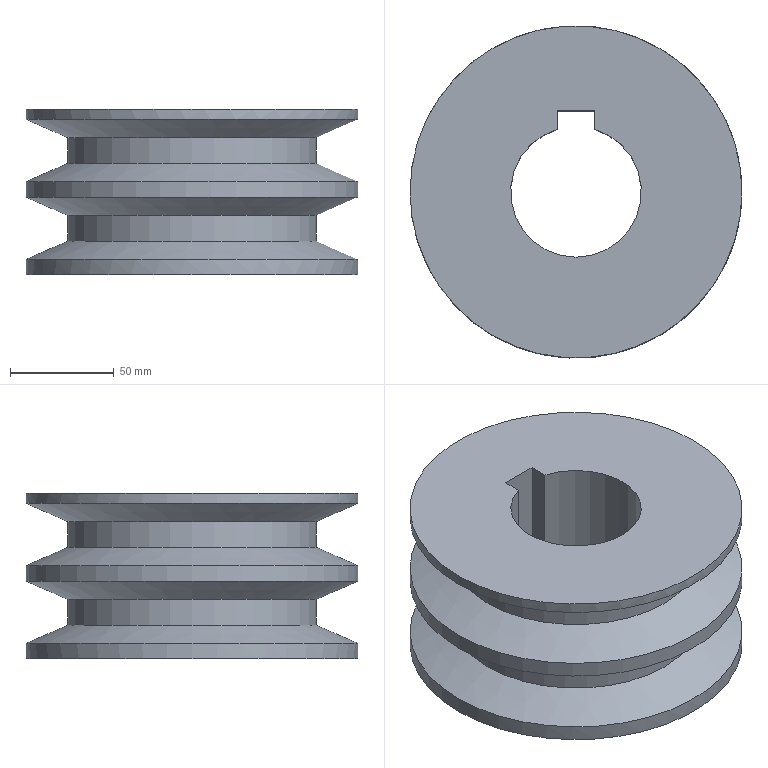Part | NX | 1 solid | 15 faces | box 160 x 160 x 80 mm | volume 966511 mm3 | cylinder 6 | plane 5 | cone 4 | commonest cylinder face diameters 160 x3 120 x2 63 x1
STEP:
#1=CARTESIAN_POINT('',(966.594,-288.856,-203.));
#2=VERTEX_POINT('',#1);
#3=CARTESIAN_POINT('',(1046.594,-288.856,-203.));
#4=DIRECTION('',(0.,0.,-1.));
#5=DIRECTION('',(-1.,0.,0.));
#6=AXIS2_PLACEMENT_3D('',#3,#4,#5);
#7=CIRCLE('',#6,80.);
#8=EDGE_CURVE('',#2,#2,#7,.T.);
#9=ORIENTED_EDGE('',*,*,#8,.F.);
#10=EDGE_LOOP('',(#9));
#11=FACE_BOUND('',#10,.T.);
#12=CARTESIAN_POINT('',(1126.594,-288.856,-198.));
#13=VERTEX_POINT('',#12);
#14=CARTESIAN_POINT('',(1046.594,-288.856,-198.));
#15=DIRECTION('',(0.,0.,-1.));
#16=DIRECTION('',(1.,0.,0.));
#17=AXIS2_PLACEMENT_3D('',#14,#15,#16);
#18=CIRCLE('',#17,80.);
#19=EDGE_CURVE('',#13,#13,#18,.T.);
#20=ORIENTED_EDGE('',*,*,#19,.T.);
#21=EDGE_LOOP('',(#20));
#22=FACE_BOUND('',#21,.T.);
#23=CARTESIAN_POINT('',(1046.594,-288.856,-278.));
#24=DIRECTION('',(0.,0.,1.));
#25=DIRECTION('',(-1.,0.,0.));
#26=AXIS2_PLACEMENT_3D('',#23,#24,#25);
#27=CYLINDRICAL_SURFACE('',#26,80.);
#28=ADVANCED_FACE('',(#11,#22),#27,.T.);
#29=CARTESIAN_POINT('',(1055.594,-258.669,-198.));
#30=VERTEX_POINT('',#29);
#31=CARTESIAN_POINT('',(1037.594,-258.669,-198.));
#32=VERTEX_POINT('',#31);
#33=CARTESIAN_POINT('',(1046.594,-288.856,-198.));
#34=DIRECTION('',(0.,0.,-1.));
#35=DIRECTION('',(-1.,0.,0.));
#36=AXIS2_PLACEMENT_3D('',#33,#34,#35);
#37=CIRCLE('',#36,31.5);
#38=EDGE_CURVE('',#30,#32,#37,.T.);
#39=ORIENTED_EDGE('',*,*,#38,.T.);
#40=CARTESIAN_POINT('',(1037.594,-249.856,-198.));
#41=VERTEX_POINT('',#40);
#42=CARTESIAN_POINT('',(1037.594,-288.856,-198.));
#43=DIRECTION('',(0.,1.,0.));
#44=VECTOR('',#43,1.);
#45=LINE('',#42,#44);
#46=EDGE_CURVE('',#32,#41,#45,.T.);
#47=ORIENTED_EDGE('',*,*,#46,.T.);
#48=CARTESIAN_POINT('',(1055.594,-249.856,-198.));
#49=VERTEX_POINT('',#48);
#50=CARTESIAN_POINT('',(1046.594,-249.856,-198.));
#51=DIRECTION('',(1.,0.,0.));
#52=VECTOR('',#51,1.);
#53=LINE('',#50,#52);
#54=EDGE_CURVE('',#41,#49,#53,.T.);
#55=ORIENTED_EDGE('',*,*,#54,.T.);
#56=CARTESIAN_POINT('',(1055.594,-288.856,-198.));
#57=DIRECTION('',(0.,-1.,0.));
#58=VECTOR('',#57,1.);
#59=LINE('',#56,#58);
#60=EDGE_CURVE('',#49,#30,#59,.T.);
#61=ORIENTED_EDGE('',*,*,#60,.T.);
#62=EDGE_LOOP('',(#39,#47,#55,#61));
#63=FACE_BOUND('',#62,.T.);
#64=ORIENTED_EDGE('',*,*,#19,.F.);
#65=EDGE_LOOP('',(#64));
#66=FACE_BOUND('',#65,.T.);
#67=CARTESIAN_POINT('',(1046.594,-288.856,-198.));
#68=DIRECTION('',(0.,0.,-1.));
#69=DIRECTION('',(1.,0.,0.));
#70=AXIS2_PLACEMENT_3D('',#67,#68,#69);
#71=PLANE('',#70);
#72=ADVANCED_FACE('',(#63,#66),#71,.F.);
#73=CARTESIAN_POINT('',(986.594,-288.856,-224.25));
#74=VERTEX_POINT('',#73);
#75=CARTESIAN_POINT('',(1046.594,-288.856,-224.25));
#76=DIRECTION('',(0.,0.,1.));
#77=DIRECTION('',(-1.,0.,0.));
#78=AXIS2_PLACEMENT_3D('',#75,#76,#77);
#79=CIRCLE('',#78,60.);
#80=EDGE_CURVE('',#74,#74,#79,.T.);
#81=ORIENTED_EDGE('',*,*,#80,.T.);
#82=EDGE_LOOP('',(#81));
#83=FACE_BOUND('',#82,.T.);
#84=CARTESIAN_POINT('',(986.594,-288.856,-211.75));
#85=VERTEX_POINT('',#84);
#86=CARTESIAN_POINT('',(1046.594,-288.856,-211.75));
#87=DIRECTION('',(0.,0.,1.));
#88=DIRECTION('',(-1.,0.,0.));
#89=AXIS2_PLACEMENT_3D('',#86,#87,#88);
#90=CIRCLE('',#89,60.);
#91=EDGE_CURVE('',#85,#85,#90,.T.);
#92=ORIENTED_EDGE('',*,*,#91,.F.);
#93=EDGE_LOOP('',(#92));
#94=FACE_BOUND('',#93,.T.);
#95=CARTESIAN_POINT('',(1046.594,-288.856,-278.));
#96=DIRECTION('',(0.,0.,-1.));
#97=DIRECTION('',(1.,0.,0.));
#98=AXIS2_PLACEMENT_3D('',#95,#96,#97);
#99=CYLINDRICAL_SURFACE('',#98,60.);
#100=ADVANCED_FACE('',(#83,#94),#99,.T.);
#101=CARTESIAN_POINT('',(966.594,-288.856,-233.));
#102=VERTEX_POINT('',#101);
#103=CARTESIAN_POINT('',(1046.594,-288.856,-233.));
#104=DIRECTION('',(0.,0.,-1.));
#105=DIRECTION('',(-1.,0.,0.));
#106=AXIS2_PLACEMENT_3D('',#103,#104,#105);
#107=CIRCLE('',#106,80.);
#108=EDGE_CURVE('',#102,#102,#107,.T.);
#109=ORIENTED_EDGE('',*,*,#108,.F.);
#110=EDGE_LOOP('',(#109));
#111=FACE_BOUND('',#110,.T.);
#112=ORIENTED_EDGE('',*,*,#80,.F.);
#113=EDGE_LOOP('',(#112));
#114=FACE_BOUND('',#113,.T.);
#115=CARTESIAN_POINT('',(1046.594,-288.856,-224.25));
#116=DIRECTION('',(0.,0.,-1.));
#117=DIRECTION('',(1.,0.,0.));
#118=AXIS2_PLACEMENT_3D('',#115,#116,#117);
#119=CONICAL_SURFACE('',#118,60.,66.371);
#120=ADVANCED_FACE('',(#111,#114),#119,.T.);
#121=ORIENTED_EDGE('',*,*,#91,.T.);
#122=EDGE_LOOP('',(#121));
#123=FACE_BOUND('',#122,.T.);
#124=ORIENTED_EDGE('',*,*,#8,.T.);
#125=EDGE_LOOP('',(#124));
#126=FACE_BOUND('',#125,.T.);
#127=CARTESIAN_POINT('',(1046.594,-288.856,-203.));
#128=DIRECTION('',(0.,0.,1.));
#129=DIRECTION('',(-1.,0.,0.));
#130=AXIS2_PLACEMENT_3D('',#127,#128,#129);
#131=CONICAL_SURFACE('',#130,80.,66.371);
#132=ADVANCED_FACE('',(#123,#126),#131,.T.);
#133=ORIENTED_EDGE('',*,*,#108,.T.);
#134=EDGE_LOOP('',(#133));
#135=FACE_BOUND('',#134,.T.);
#136=CARTESIAN_POINT('',(966.594,-288.856,-240.5));
#137=VERTEX_POINT('',#136);
#138=CARTESIAN_POINT('',(1046.594,-288.856,-240.5));
#139=DIRECTION('',(0.,0.,-1.));
#140=DIRECTION('',(-1.,0.,0.));
#141=AXIS2_PLACEMENT_3D('',#138,#139,#140);
#142=CIRCLE('',#141,80.);
#143=EDGE_CURVE('',#137,#137,#142,.T.);
#144=ORIENTED_EDGE('',*,*,#143,.F.);
#145=EDGE_LOOP('',(#144));
#146=FACE_BOUND('',#145,.T.);
#147=CARTESIAN_POINT('',(1046.594,-288.856,-278.));
#148=DIRECTION('',(0.,0.,1.));
#149=DIRECTION('',(-1.,0.,0.));
#150=AXIS2_PLACEMENT_3D('',#147,#148,#149);
#151=CYLINDRICAL_SURFACE('',#150,80.);
#152=ADVANCED_FACE('',(#135,#146),#151,.T.);
#153=CARTESIAN_POINT('',(986.594,-288.856,-261.75));
#154=VERTEX_POINT('',#153);
#155=CARTESIAN_POINT('',(1046.594,-288.856,-261.75));
#156=DIRECTION('',(0.,0.,1.));
#157=DIRECTION('',(-1.,0.,0.));
#158=AXIS2_PLACEMENT_3D('',#155,#156,#157);
#159=CIRCLE('',#158,60.);
#160=EDGE_CURVE('',#154,#154,#159,.T.);
#161=ORIENTED_EDGE('',*,*,#160,.T.);
#162=EDGE_LOOP('',(#161));
#163=FACE_BOUND('',#162,.T.);
#164=CARTESIAN_POINT('',(986.594,-288.856,-249.25));
#165=VERTEX_POINT('',#164);
#166=CARTESIAN_POINT('',(1046.594,-288.856,-249.25));
#167=DIRECTION('',(0.,0.,1.));
#168=DIRECTION('',(-1.,0.,0.));
#169=AXIS2_PLACEMENT_3D('',#166,#167,#168);
#170=CIRCLE('',#169,60.);
#171=EDGE_CURVE('',#165,#165,#170,.T.);
#172=ORIENTED_EDGE('',*,*,#171,.F.);
#173=EDGE_LOOP('',(#172));
#174=FACE_BOUND('',#173,.T.);
#175=CARTESIAN_POINT('',(1046.594,-288.856,-278.));
#176=DIRECTION('',(0.,0.,-1.));
#177=DIRECTION('',(1.,0.,0.));
#178=AXIS2_PLACEMENT_3D('',#175,#176,#177);
#179=CYLINDRICAL_SURFACE('',#178,60.);
#180=ADVANCED_FACE('',(#163,#174),#179,.T.);
#181=CARTESIAN_POINT('',(966.594,-288.856,-270.5));
#182=VERTEX_POINT('',#181);
#183=CARTESIAN_POINT('',(1046.594,-288.856,-270.5));
#184=DIRECTION('',(0.,0.,-1.));
#185=DIRECTION('',(-1.,0.,0.));
#186=AXIS2_PLACEMENT_3D('',#183,#184,#185);
#187=CIRCLE('',#186,80.);
#188=EDGE_CURVE('',#182,#182,#187,.T.);
#189=ORIENTED_EDGE('',*,*,#188,.F.);
#190=EDGE_LOOP('',(#189));
#191=FACE_BOUND('',#190,.T.);
#192=ORIENTED_EDGE('',*,*,#160,.F.);
#193=EDGE_LOOP('',(#192));
#194=FACE_BOUND('',#193,.T.);
#195=CARTESIAN_POINT('',(1046.594,-288.856,-261.75));
#196=DIRECTION('',(0.,0.,-1.));
#197=DIRECTION('',(1.,0.,0.));
#198=AXIS2_PLACEMENT_3D('',#195,#196,#197);
#199=CONICAL_SURFACE('',#198,60.,66.371);
#200=ADVANCED_FACE('',(#191,#194),#199,.T.);
#201=ORIENTED_EDGE('',*,*,#171,.T.);
#202=EDGE_LOOP('',(#201));
#203=FACE_BOUND('',#202,.T.);
#204=ORIENTED_EDGE('',*,*,#143,.T.);
#205=EDGE_LOOP('',(#204));
#206=FACE_BOUND('',#205,.T.);
#207=CARTESIAN_POINT('',(1046.594,-288.856,-240.5));
#208=DIRECTION('',(0.,0.,1.));
#209=DIRECTION('',(-1.,0.,0.));
#210=AXIS2_PLACEMENT_3D('',#207,#208,#209);
#211=CONICAL_SURFACE('',#210,80.,66.371);
#212=ADVANCED_FACE('',(#203,#206),#211,.T.);
#213=CARTESIAN_POINT('',(1037.594,-258.669,-278.));
#214=VERTEX_POINT('',#213);
#215=CARTESIAN_POINT('',(1037.594,-249.856,-278.));
#216=VERTEX_POINT('',#215);
#217=CARTESIAN_POINT('',(1037.594,-279.856,-278.));
#218=DIRECTION('',(0.,1.,0.));
#219=VECTOR('',#218,1.);
#220=LINE('',#217,#219);
#221=EDGE_CURVE('',#214,#216,#220,.T.);
#222=ORIENTED_EDGE('',*,*,#221,.F.);
#223=CARTESIAN_POINT('',(1055.594,-258.669,-278.));
#224=VERTEX_POINT('',#223);
#225=CARTESIAN_POINT('',(1046.594,-288.856,-278.));
#226=DIRECTION('',(0.,0.,-1.));
#227=DIRECTION('',(-1.,0.,0.));
#228=AXIS2_PLACEMENT_3D('',#225,#226,#227);
#229=CIRCLE('',#228,31.5);
#230=EDGE_CURVE('',#224,#214,#229,.T.);
#231=ORIENTED_EDGE('',*,*,#230,.F.);
#232=CARTESIAN_POINT('',(1055.594,-249.856,-278.));
#233=VERTEX_POINT('',#232);
#234=CARTESIAN_POINT('',(1055.594,-249.856,-278.));
#235=DIRECTION('',(0.,-1.,0.));
#236=VECTOR('',#235,1.);
#237=LINE('',#234,#236);
#238=EDGE_CURVE('',#233,#224,#237,.T.);
#239=ORIENTED_EDGE('',*,*,#238,.F.);
#240=CARTESIAN_POINT('',(1037.594,-249.856,-278.));
#241=DIRECTION('',(1.,0.,0.));
#242=VECTOR('',#241,1.);
#243=LINE('',#240,#242);
#244=EDGE_CURVE('',#216,#233,#243,.T.);
#245=ORIENTED_EDGE('',*,*,#244,.F.);
#246=EDGE_LOOP('',(#222,#231,#239,#245));
#247=FACE_BOUND('',#246,.T.);
#248=CARTESIAN_POINT('',(1126.594,-288.856,-278.));
#249=VERTEX_POINT('',#248);
#250=CARTESIAN_POINT('',(1046.594,-288.856,-278.));
#251=DIRECTION('',(0.,0.,-1.));
#252=DIRECTION('',(1.,0.,0.));
#253=AXIS2_PLACEMENT_3D('',#250,#251,#252);
#254=CIRCLE('',#253,80.);
#255=EDGE_CURVE('',#249,#249,#254,.T.);
#256=ORIENTED_EDGE('',*,*,#255,.T.);
#257=EDGE_LOOP('',(#256));
#258=FACE_BOUND('',#257,.T.);
#259=CARTESIAN_POINT('',(1046.594,-288.856,-278.));
#260=DIRECTION('',(0.,0.,-1.));
#261=DIRECTION('',(1.,0.,0.));
#262=AXIS2_PLACEMENT_3D('',#259,#260,#261);
#263=PLANE('',#262);
#264=ADVANCED_FACE('',(#247,#258),#263,.T.);
#265=ORIENTED_EDGE('',*,*,#188,.T.);
#266=EDGE_LOOP('',(#265));
#267=FACE_BOUND('',#266,.T.);
#268=ORIENTED_EDGE('',*,*,#255,.F.);
#269=EDGE_LOOP('',(#268));
#270=FACE_BOUND('',#269,.T.);
#271=CARTESIAN_POINT('',(1046.594,-288.856,-278.));
#272=DIRECTION('',(0.,0.,1.));
#273=DIRECTION('',(-1.,0.,0.));
#274=AXIS2_PLACEMENT_3D('',#271,#272,#273);
#275=CYLINDRICAL_SURFACE('',#274,80.);
#276=ADVANCED_FACE('',(#267,#270),#275,.T.);
#277=ORIENTED_EDGE('',*,*,#230,.T.);
#278=CARTESIAN_POINT('',(1037.594,-258.669,-335.));
#279=DIRECTION('',(0.,0.,1.));
#280=VECTOR('',#279,1.);
#281=LINE('',#278,#280);
#282=EDGE_CURVE('',#214,#32,#281,.T.);
#283=ORIENTED_EDGE('',*,*,#282,.T.);
#284=ORIENTED_EDGE('',*,*,#38,.F.);
#285=CARTESIAN_POINT('',(1055.594,-258.669,-335.));
#286=DIRECTION('',(0.,0.,-1.));
#287=VECTOR('',#286,1.);
#288=LINE('',#285,#287);
#289=EDGE_CURVE('',#30,#224,#288,.T.);
#290=ORIENTED_EDGE('',*,*,#289,.T.);
#291=EDGE_LOOP('',(#277,#283,#284,#290));
#292=FACE_OUTER_BOUND('',#291,.T.);
#293=CARTESIAN_POINT('',(1046.594,-288.856,-335.));
#294=DIRECTION('',(0.,0.,1.));
#295=DIRECTION('',(-1.,0.,0.));
#296=AXIS2_PLACEMENT_3D('',#293,#294,#295);
#297=CYLINDRICAL_SURFACE('',#296,31.5);
#298=ADVANCED_FACE('',(#292),#297,.F.);
#299=CARTESIAN_POINT('',(1037.594,-249.856,-158.));
#300=DIRECTION('',(0.,0.,1.));
#301=VECTOR('',#300,1.);
#302=LINE('',#299,#301);
#303=EDGE_CURVE('',#216,#41,#302,.T.);
#304=ORIENTED_EDGE('',*,*,#303,.F.);
#305=ORIENTED_EDGE('',*,*,#244,.T.);
#306=CARTESIAN_POINT('',(1055.594,-249.856,-158.));
#307=DIRECTION('',(0.,0.,1.));
#308=VECTOR('',#307,1.);
#309=LINE('',#306,#308);
#310=EDGE_CURVE('',#233,#49,#309,.T.);
#311=ORIENTED_EDGE('',*,*,#310,.T.);
#312=ORIENTED_EDGE('',*,*,#54,.F.);
#313=EDGE_LOOP('',(#304,#305,#311,#312));
#314=FACE_OUTER_BOUND('',#313,.T.);
#315=CARTESIAN_POINT('',(1037.594,-249.856,-158.));
#316=DIRECTION('',(0.,1.,0.));
#317=DIRECTION('',(0.,0.,-1.));
#318=AXIS2_PLACEMENT_3D('',#315,#316,#317);
#319=PLANE('',#318);
#320=ADVANCED_FACE('',(#314),#319,.F.);
#321=ORIENTED_EDGE('',*,*,#282,.F.);
#322=ORIENTED_EDGE('',*,*,#221,.T.);
#323=ORIENTED_EDGE('',*,*,#303,.T.);
#324=ORIENTED_EDGE('',*,*,#46,.F.);
#325=EDGE_LOOP('',(#321,#322,#323,#324));
#326=FACE_OUTER_BOUND('',#325,.T.);
#327=CARTESIAN_POINT('',(1037.594,-279.856,-158.));
#328=DIRECTION('',(-1.,0.,0.));
#329=DIRECTION('',(0.,0.,-1.));
#330=AXIS2_PLACEMENT_3D('',#327,#328,#329);
#331=PLANE('',#330);
#332=ADVANCED_FACE('',(#326),#331,.F.);
#333=ORIENTED_EDGE('',*,*,#310,.F.);
#334=ORIENTED_EDGE('',*,*,#238,.T.);
#335=ORIENTED_EDGE('',*,*,#289,.F.);
#336=ORIENTED_EDGE('',*,*,#60,.F.);
#337=EDGE_LOOP('',(#333,#334,#335,#336));
#338=FACE_OUTER_BOUND('',#337,.T.);
#339=CARTESIAN_POINT('',(1055.594,-249.856,-158.));
#340=DIRECTION('',(1.,0.,0.));
#341=DIRECTION('',(0.,0.,1.));
#342=AXIS2_PLACEMENT_3D('',#339,#340,#341);
#343=PLANE('',#342);
#344=ADVANCED_FACE('',(#338),#343,.F.);
#345=CLOSED_SHELL('',(#28,#72,#100,#120,#132,#152,#180,#200,#212,#264,#276,#298,#320,#332,#344));
#346=MANIFOLD_SOLID_BREP('',#345);
#347=(LENGTH_UNIT()NAMED_UNIT(*)SI_UNIT(.MILLI.,.METRE.));
#348=UNCERTAINTY_MEASURE_WITH_UNIT(LENGTH_MEASURE(0.00002),#347,'','');
#349=(NAMED_UNIT(*)PLANE_ANGLE_UNIT()SI_UNIT($,.RADIAN.));
#350=PLANE_ANGLE_MEASURE_WITH_UNIT(PLANE_ANGLE_MEASURE(0.01745),#349);
#351=DIMENSIONAL_EXPONENTS(0.,0.,0.,0.,0.,0.,0.);
#352=(CONVERSION_BASED_UNIT('DEGREE',#350)NAMED_UNIT(#351)PLANE_ANGLE_UNIT());
#353=(NAMED_UNIT(*)SI_UNIT($,.STERADIAN.)SOLID_ANGLE_UNIT());
#354=(GEOMETRIC_REPRESENTATION_CONTEXT(3)GLOBAL_UNCERTAINTY_ASSIGNED_CONTEXT((#348))GLOBAL_UNIT_ASSIGNED_CONTEXT((#347,#352,#353))REPRESENTATION_CONTEXT('',''));
#355=ADVANCED_BREP_SHAPE_REPRESENTATION('',(#346),#354);